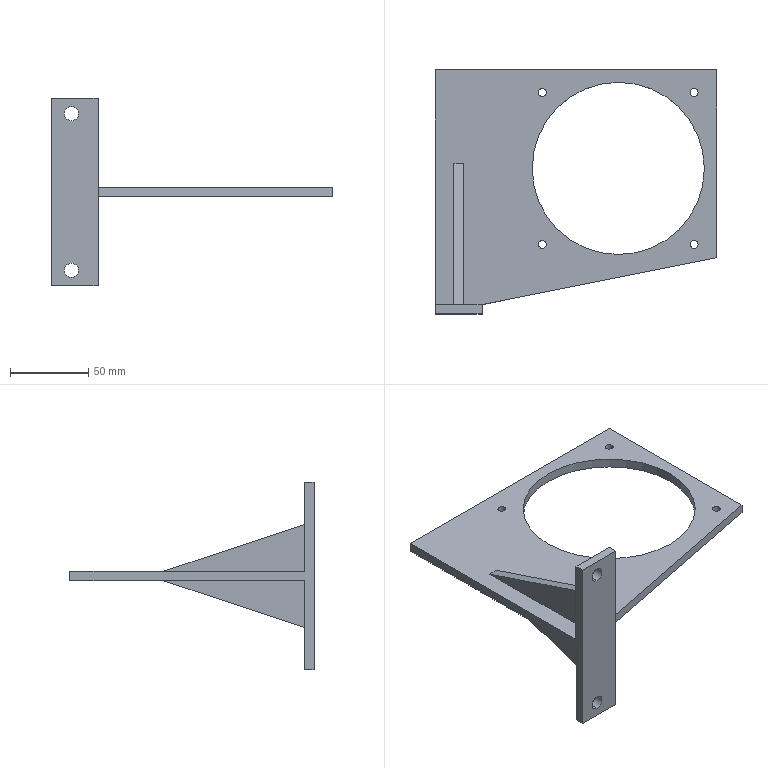Part | SolidWorks | features ICE 3, Extrusion 1 | 1 solid | 32 faces | box 180 x 156 x 120 mm | volume 128045 mm3 | plane 18 | cylinder 14 | commonest cylinder face diameters 5 x8 9 x4 110 x2
STEP:
#1=CARTESIAN_POINT('',(13.,-6.,48.5));
#2=VERTEX_POINT('',#1);
#3=CARTESIAN_POINT('',(13.,-6.,57.5));
#4=VERTEX_POINT('',#3);
#5=CARTESIAN_POINT('',(13.,-6.,53.));
#6=DIRECTION('',(0.,1.,0.));
#7=DIRECTION('',(0.,0.,1.));
#8=AXIS2_PLACEMENT_3D('',#5,#6,#7);
#9=CIRCLE('',#8,4.5);
#10=EDGE_CURVE('',#2,#4,#9,.T.);
#11=ORIENTED_EDGE('',*,*,#10,.F.);
#12=CARTESIAN_POINT('',(13.,0.,48.5));
#13=VERTEX_POINT('',#12);
#14=CARTESIAN_POINT('',(13.,-6.,48.5));
#15=DIRECTION('',(0.,1.,0.));
#16=VECTOR('',#15,1000.);
#17=LINE('',#14,#16);
#18=EDGE_CURVE('',#2,#13,#17,.T.);
#19=ORIENTED_EDGE('',*,*,#18,.T.);
#20=CARTESIAN_POINT('',(13.,0.,57.5));
#21=VERTEX_POINT('',#20);
#22=CARTESIAN_POINT('',(13.,0.,53.));
#23=DIRECTION('',(0.,1.,0.));
#24=DIRECTION('',(0.,0.,1.));
#25=AXIS2_PLACEMENT_3D('',#22,#23,#24);
#26=CIRCLE('',#25,4.5);
#27=EDGE_CURVE('',#13,#21,#26,.T.);
#28=ORIENTED_EDGE('',*,*,#27,.T.);
#29=CARTESIAN_POINT('',(13.,-6.,57.5));
#30=DIRECTION('',(0.,1.,0.));
#31=VECTOR('',#30,1000.);
#32=LINE('',#29,#31);
#33=EDGE_CURVE('',#4,#21,#32,.T.);
#34=ORIENTED_EDGE('',*,*,#33,.F.);
#35=EDGE_LOOP('',(#11,#19,#28,#34));
#36=FACE_OUTER_BOUND('',#35,.T.);
#37=CARTESIAN_POINT('',(13.,-6.,53.));
#38=DIRECTION('',(0.,1.,0.));
#39=DIRECTION('',(0.,0.,1.));
#40=AXIS2_PLACEMENT_3D('',#37,#38,#39);
#41=CYLINDRICAL_SURFACE('',#40,4.5);
#42=ADVANCED_FACE('',(#36),#41,.F.);
#43=CARTESIAN_POINT('',(13.,-6.,-51.5));
#44=VERTEX_POINT('',#43);
#45=CARTESIAN_POINT('',(13.,-6.,-42.5));
#46=VERTEX_POINT('',#45);
#47=CARTESIAN_POINT('',(13.,-6.,-47.));
#48=DIRECTION('',(0.,1.,0.));
#49=DIRECTION('',(0.,0.,1.));
#50=AXIS2_PLACEMENT_3D('',#47,#48,#49);
#51=CIRCLE('',#50,4.5);
#52=EDGE_CURVE('',#44,#46,#51,.T.);
#53=ORIENTED_EDGE('',*,*,#52,.F.);
#54=CARTESIAN_POINT('',(13.,0.,-51.5));
#55=VERTEX_POINT('',#54);
#56=CARTESIAN_POINT('',(13.,-6.,-51.5));
#57=DIRECTION('',(0.,1.,0.));
#58=VECTOR('',#57,1000.);
#59=LINE('',#56,#58);
#60=EDGE_CURVE('',#44,#55,#59,.T.);
#61=ORIENTED_EDGE('',*,*,#60,.T.);
#62=CARTESIAN_POINT('',(13.,0.,-42.5));
#63=VERTEX_POINT('',#62);
#64=CARTESIAN_POINT('',(13.,0.,-47.));
#65=DIRECTION('',(0.,1.,0.));
#66=DIRECTION('',(0.,0.,1.));
#67=AXIS2_PLACEMENT_3D('',#64,#65,#66);
#68=CIRCLE('',#67,4.5);
#69=EDGE_CURVE('',#55,#63,#68,.T.);
#70=ORIENTED_EDGE('',*,*,#69,.T.);
#71=CARTESIAN_POINT('',(13.,-6.,-42.5));
#72=DIRECTION('',(0.,1.,0.));
#73=VECTOR('',#72,1000.);
#74=LINE('',#71,#73);
#75=EDGE_CURVE('',#46,#63,#74,.T.);
#76=ORIENTED_EDGE('',*,*,#75,.F.);
#77=EDGE_LOOP('',(#53,#61,#70,#76));
#78=FACE_OUTER_BOUND('',#77,.T.);
#79=CARTESIAN_POINT('',(13.,-6.,-47.));
#80=DIRECTION('',(0.,1.,0.));
#81=DIRECTION('',(0.,0.,1.));
#82=AXIS2_PLACEMENT_3D('',#79,#80,#81);
#83=CYLINDRICAL_SURFACE('',#82,4.5);
#84=ADVANCED_FACE('',(#78),#83,.F.);
#85=CARTESIAN_POINT('',(62.,87.,6.));
#86=VERTEX_POINT('',#85);
#87=CARTESIAN_POINT('',(172.,87.,6.));
#88=VERTEX_POINT('',#87);
#89=CARTESIAN_POINT('',(117.,87.,6.));
#90=DIRECTION('',(0.,0.,1.));
#91=DIRECTION('',(1.,0.,0.));
#92=AXIS2_PLACEMENT_3D('',#89,#90,#91);
#93=CIRCLE('',#92,55.);
#94=EDGE_CURVE('',#86,#88,#93,.T.);
#95=ORIENTED_EDGE('',*,*,#94,.T.);
#96=CARTESIAN_POINT('',(172.,87.,0.));
#97=VERTEX_POINT('',#96);
#98=CARTESIAN_POINT('',(172.,87.,6.));
#99=DIRECTION('',(0.,0.,-1.));
#100=VECTOR('',#99,1000.);
#101=LINE('',#98,#100);
#102=EDGE_CURVE('',#88,#97,#101,.T.);
#103=ORIENTED_EDGE('',*,*,#102,.T.);
#104=CARTESIAN_POINT('',(62.,87.,0.));
#105=VERTEX_POINT('',#104);
#106=CARTESIAN_POINT('',(117.,87.,0.));
#107=DIRECTION('',(0.,0.,1.));
#108=DIRECTION('',(1.,0.,0.));
#109=AXIS2_PLACEMENT_3D('',#106,#107,#108);
#110=CIRCLE('',#109,55.);
#111=EDGE_CURVE('',#105,#97,#110,.T.);
#112=ORIENTED_EDGE('',*,*,#111,.F.);
#113=CARTESIAN_POINT('',(62.,87.,6.));
#114=DIRECTION('',(0.,0.,-1.));
#115=VECTOR('',#114,1000.);
#116=LINE('',#113,#115);
#117=EDGE_CURVE('',#86,#105,#116,.T.);
#118=ORIENTED_EDGE('',*,*,#117,.F.);
#119=EDGE_LOOP('',(#95,#103,#112,#118));
#120=FACE_OUTER_BOUND('',#119,.T.);
#121=CARTESIAN_POINT('',(117.,87.,6.));
#122=DIRECTION('',(0.,0.,-1.));
#123=DIRECTION('',(-1.,0.,0.));
#124=AXIS2_PLACEMENT_3D('',#121,#122,#123);
#125=CYLINDRICAL_SURFACE('',#124,55.);
#126=ADVANCED_FACE('',(#120),#125,.F.);
#127=CARTESIAN_POINT('',(66.,38.5,6.));
#128=VERTEX_POINT('',#127);
#129=CARTESIAN_POINT('',(71.,38.5,6.));
#130=VERTEX_POINT('',#129);
#131=CARTESIAN_POINT('',(68.5,38.5,6.));
#132=DIRECTION('',(0.,0.,1.));
#133=DIRECTION('',(1.,0.,0.));
#134=AXIS2_PLACEMENT_3D('',#131,#132,#133);
#135=CIRCLE('',#134,2.5);
#136=EDGE_CURVE('',#128,#130,#135,.T.);
#137=ORIENTED_EDGE('',*,*,#136,.T.);
#138=CARTESIAN_POINT('',(71.,38.5,0.));
#139=VERTEX_POINT('',#138);
#140=CARTESIAN_POINT('',(71.,38.5,6.));
#141=DIRECTION('',(0.,0.,-1.));
#142=VECTOR('',#141,1000.);
#143=LINE('',#140,#142);
#144=EDGE_CURVE('',#130,#139,#143,.T.);
#145=ORIENTED_EDGE('',*,*,#144,.T.);
#146=CARTESIAN_POINT('',(66.,38.5,0.));
#147=VERTEX_POINT('',#146);
#148=CARTESIAN_POINT('',(68.5,38.5,0.));
#149=DIRECTION('',(0.,0.,1.));
#150=DIRECTION('',(1.,0.,0.));
#151=AXIS2_PLACEMENT_3D('',#148,#149,#150);
#152=CIRCLE('',#151,2.5);
#153=EDGE_CURVE('',#147,#139,#152,.T.);
#154=ORIENTED_EDGE('',*,*,#153,.F.);
#155=CARTESIAN_POINT('',(66.,38.5,6.));
#156=DIRECTION('',(0.,0.,-1.));
#157=VECTOR('',#156,1000.);
#158=LINE('',#155,#157);
#159=EDGE_CURVE('',#128,#147,#158,.T.);
#160=ORIENTED_EDGE('',*,*,#159,.F.);
#161=EDGE_LOOP('',(#137,#145,#154,#160));
#162=FACE_OUTER_BOUND('',#161,.T.);
#163=CARTESIAN_POINT('',(68.5,38.5,6.));
#164=DIRECTION('',(0.,0.,-1.));
#165=DIRECTION('',(-1.,0.,0.));
#166=AXIS2_PLACEMENT_3D('',#163,#164,#165);
#167=CYLINDRICAL_SURFACE('',#166,2.5);
#168=ADVANCED_FACE('',(#162),#167,.F.);
#169=CARTESIAN_POINT('',(163.,38.5,6.));
#170=VERTEX_POINT('',#169);
#171=CARTESIAN_POINT('',(168.,38.5,6.));
#172=VERTEX_POINT('',#171);
#173=CARTESIAN_POINT('',(165.5,38.5,6.));
#174=DIRECTION('',(0.,0.,1.));
#175=DIRECTION('',(1.,0.,0.));
#176=AXIS2_PLACEMENT_3D('',#173,#174,#175);
#177=CIRCLE('',#176,2.5);
#178=EDGE_CURVE('',#170,#172,#177,.T.);
#179=ORIENTED_EDGE('',*,*,#178,.T.);
#180=CARTESIAN_POINT('',(168.,38.5,0.));
#181=VERTEX_POINT('',#180);
#182=CARTESIAN_POINT('',(168.,38.5,6.));
#183=DIRECTION('',(0.,0.,-1.));
#184=VECTOR('',#183,1000.);
#185=LINE('',#182,#184);
#186=EDGE_CURVE('',#172,#181,#185,.T.);
#187=ORIENTED_EDGE('',*,*,#186,.T.);
#188=CARTESIAN_POINT('',(163.,38.5,0.));
#189=VERTEX_POINT('',#188);
#190=CARTESIAN_POINT('',(165.5,38.5,0.));
#191=DIRECTION('',(0.,0.,1.));
#192=DIRECTION('',(1.,0.,0.));
#193=AXIS2_PLACEMENT_3D('',#190,#191,#192);
#194=CIRCLE('',#193,2.5);
#195=EDGE_CURVE('',#189,#181,#194,.T.);
#196=ORIENTED_EDGE('',*,*,#195,.F.);
#197=CARTESIAN_POINT('',(163.,38.5,6.));
#198=DIRECTION('',(0.,0.,-1.));
#199=VECTOR('',#198,1000.);
#200=LINE('',#197,#199);
#201=EDGE_CURVE('',#170,#189,#200,.T.);
#202=ORIENTED_EDGE('',*,*,#201,.F.);
#203=EDGE_LOOP('',(#179,#187,#196,#202));
#204=FACE_OUTER_BOUND('',#203,.T.);
#205=CARTESIAN_POINT('',(165.5,38.5,6.));
#206=DIRECTION('',(0.,0.,-1.));
#207=DIRECTION('',(-1.,0.,0.));
#208=AXIS2_PLACEMENT_3D('',#205,#206,#207);
#209=CYLINDRICAL_SURFACE('',#208,2.5);
#210=ADVANCED_FACE('',(#204),#209,.F.);
#211=CARTESIAN_POINT('',(66.,135.5,6.));
#212=VERTEX_POINT('',#211);
#213=CARTESIAN_POINT('',(71.,135.5,6.));
#214=VERTEX_POINT('',#213);
#215=CARTESIAN_POINT('',(68.5,135.5,6.));
#216=DIRECTION('',(0.,0.,1.));
#217=DIRECTION('',(1.,0.,0.));
#218=AXIS2_PLACEMENT_3D('',#215,#216,#217);
#219=CIRCLE('',#218,2.5);
#220=EDGE_CURVE('',#212,#214,#219,.T.);
#221=ORIENTED_EDGE('',*,*,#220,.T.);
#222=CARTESIAN_POINT('',(71.,135.5,0.));
#223=VERTEX_POINT('',#222);
#224=CARTESIAN_POINT('',(71.,135.5,6.));
#225=DIRECTION('',(0.,0.,-1.));
#226=VECTOR('',#225,1000.);
#227=LINE('',#224,#226);
#228=EDGE_CURVE('',#214,#223,#227,.T.);
#229=ORIENTED_EDGE('',*,*,#228,.T.);
#230=CARTESIAN_POINT('',(66.,135.5,0.));
#231=VERTEX_POINT('',#230);
#232=CARTESIAN_POINT('',(68.5,135.5,0.));
#233=DIRECTION('',(0.,0.,1.));
#234=DIRECTION('',(1.,0.,0.));
#235=AXIS2_PLACEMENT_3D('',#232,#233,#234);
#236=CIRCLE('',#235,2.5);
#237=EDGE_CURVE('',#231,#223,#236,.T.);
#238=ORIENTED_EDGE('',*,*,#237,.F.);
#239=CARTESIAN_POINT('',(66.,135.5,6.));
#240=DIRECTION('',(0.,0.,-1.));
#241=VECTOR('',#240,1000.);
#242=LINE('',#239,#241);
#243=EDGE_CURVE('',#212,#231,#242,.T.);
#244=ORIENTED_EDGE('',*,*,#243,.F.);
#245=EDGE_LOOP('',(#221,#229,#238,#244));
#246=FACE_OUTER_BOUND('',#245,.T.);
#247=CARTESIAN_POINT('',(68.5,135.5,6.));
#248=DIRECTION('',(0.,0.,-1.));
#249=DIRECTION('',(-1.,0.,0.));
#250=AXIS2_PLACEMENT_3D('',#247,#248,#249);
#251=CYLINDRICAL_SURFACE('',#250,2.5);
#252=ADVANCED_FACE('',(#246),#251,.F.);
#253=CARTESIAN_POINT('',(163.,135.5,6.));
#254=VERTEX_POINT('',#253);
#255=CARTESIAN_POINT('',(168.,135.5,6.));
#256=VERTEX_POINT('',#255);
#257=CARTESIAN_POINT('',(165.5,135.5,6.));
#258=DIRECTION('',(0.,0.,1.));
#259=DIRECTION('',(1.,0.,0.));
#260=AXIS2_PLACEMENT_3D('',#257,#258,#259);
#261=CIRCLE('',#260,2.5);
#262=EDGE_CURVE('',#254,#256,#261,.T.);
#263=ORIENTED_EDGE('',*,*,#262,.T.);
#264=CARTESIAN_POINT('',(168.,135.5,0.));
#265=VERTEX_POINT('',#264);
#266=CARTESIAN_POINT('',(168.,135.5,6.));
#267=DIRECTION('',(0.,0.,-1.));
#268=VECTOR('',#267,1000.);
#269=LINE('',#266,#268);
#270=EDGE_CURVE('',#256,#265,#269,.T.);
#271=ORIENTED_EDGE('',*,*,#270,.T.);
#272=CARTESIAN_POINT('',(163.,135.5,0.));
#273=VERTEX_POINT('',#272);
#274=CARTESIAN_POINT('',(165.5,135.5,0.));
#275=DIRECTION('',(0.,0.,1.));
#276=DIRECTION('',(1.,0.,0.));
#277=AXIS2_PLACEMENT_3D('',#274,#275,#276);
#278=CIRCLE('',#277,2.5);
#279=EDGE_CURVE('',#273,#265,#278,.T.);
#280=ORIENTED_EDGE('',*,*,#279,.F.);
#281=CARTESIAN_POINT('',(163.,135.5,6.));
#282=DIRECTION('',(0.,0.,-1.));
#283=VECTOR('',#282,1000.);
#284=LINE('',#281,#283);
#285=EDGE_CURVE('',#254,#273,#284,.T.);
#286=ORIENTED_EDGE('',*,*,#285,.F.);
#287=EDGE_LOOP('',(#263,#271,#280,#286));
#288=FACE_OUTER_BOUND('',#287,.T.);
#289=CARTESIAN_POINT('',(165.5,135.5,6.));
#290=DIRECTION('',(0.,0.,-1.));
#291=DIRECTION('',(-1.,0.,0.));
#292=AXIS2_PLACEMENT_3D('',#289,#290,#291);
#293=CYLINDRICAL_SURFACE('',#292,2.5);
#294=ADVANCED_FACE('',(#288),#293,.F.);
#295=ORIENTED_EDGE('',*,*,#136,.F.);
#296=CARTESIAN_POINT('',(68.5,38.5,6.));
#297=DIRECTION('',(0.,0.,1.));
#298=DIRECTION('',(1.,0.,0.));
#299=AXIS2_PLACEMENT_3D('',#296,#297,#298);
#300=CIRCLE('',#299,2.5);
#301=EDGE_CURVE('',#130,#128,#300,.T.);
#302=ORIENTED_EDGE('',*,*,#301,.F.);
#303=EDGE_LOOP('',(#295,#302));
#304=FACE_BOUND('',#303,.T.);
#305=ORIENTED_EDGE('',*,*,#220,.F.);
#306=CARTESIAN_POINT('',(68.5,135.5,6.));
#307=DIRECTION('',(0.,0.,1.));
#308=DIRECTION('',(1.,0.,0.));
#309=AXIS2_PLACEMENT_3D('',#306,#307,#308);
#310=CIRCLE('',#309,2.5);
#311=EDGE_CURVE('',#214,#212,#310,.T.);
#312=ORIENTED_EDGE('',*,*,#311,.F.);
#313=EDGE_LOOP('',(#305,#312));
#314=FACE_BOUND('',#313,.T.);
#315=CARTESIAN_POINT('',(18.,90.,6.));
#316=VERTEX_POINT('',#315);
#317=CARTESIAN_POINT('',(12.,90.,6.));
#318=VERTEX_POINT('',#317);
#319=CARTESIAN_POINT('',(18.,90.,6.));
#320=DIRECTION('',(-1.,0.,0.));
#321=VECTOR('',#320,1000.);
#322=LINE('',#319,#321);
#323=EDGE_CURVE('',#316,#318,#322,.T.);
#324=ORIENTED_EDGE('',*,*,#323,.F.);
#325=CARTESIAN_POINT('',(18.,0.,6.));
#326=VERTEX_POINT('',#325);
#327=CARTESIAN_POINT('',(18.,0.,6.));
#328=DIRECTION('',(0.,-1.,0.));
#329=VECTOR('',#328,1000.);
#330=LINE('',#327,#329);
#331=EDGE_CURVE('',#316,#326,#330,.T.);
#332=ORIENTED_EDGE('',*,*,#331,.T.);
#333=CARTESIAN_POINT('',(30.,0.,6.));
#334=VERTEX_POINT('',#333);
#335=CARTESIAN_POINT('',(0.,0.,6.));
#336=DIRECTION('',(1.,0.,0.));
#337=VECTOR('',#336,1000.);
#338=LINE('',#335,#337);
#339=EDGE_CURVE('',#326,#334,#338,.T.);
#340=ORIENTED_EDGE('',*,*,#339,.T.);
#341=CARTESIAN_POINT('',(180.,30.,6.));
#342=VERTEX_POINT('',#341);
#343=CARTESIAN_POINT('',(180.,30.,6.));
#344=DIRECTION('',(0.9806,0.1961,0.));
#345=VECTOR('',#344,1000.);
#346=LINE('',#343,#345);
#347=EDGE_CURVE('',#334,#342,#346,.T.);
#348=ORIENTED_EDGE('',*,*,#347,.T.);
#349=CARTESIAN_POINT('',(180.,150.,6.));
#350=VERTEX_POINT('',#349);
#351=CARTESIAN_POINT('',(180.,30.,6.));
#352=DIRECTION('',(0.,1.,0.));
#353=VECTOR('',#352,1000.);
#354=LINE('',#351,#353);
#355=EDGE_CURVE('',#342,#350,#354,.T.);
#356=ORIENTED_EDGE('',*,*,#355,.T.);
#357=CARTESIAN_POINT('',(0.,150.,6.));
#358=VERTEX_POINT('',#357);
#359=CARTESIAN_POINT('',(0.,150.,6.));
#360=DIRECTION('',(-1.,0.,0.));
#361=VECTOR('',#360,1000.);
#362=LINE('',#359,#361);
#363=EDGE_CURVE('',#350,#358,#362,.T.);
#364=ORIENTED_EDGE('',*,*,#363,.T.);
#365=CARTESIAN_POINT('',(0.,0.,6.));
#366=VERTEX_POINT('',#365);
#367=CARTESIAN_POINT('',(0.,0.,6.));
#368=DIRECTION('',(0.,-1.,0.));
#369=VECTOR('',#368,1000.);
#370=LINE('',#367,#369);
#371=EDGE_CURVE('',#358,#366,#370,.T.);
#372=ORIENTED_EDGE('',*,*,#371,.T.);
#373=CARTESIAN_POINT('',(12.,0.,6.));
#374=VERTEX_POINT('',#373);
#375=CARTESIAN_POINT('',(0.,0.,6.));
#376=DIRECTION('',(1.,0.,0.));
#377=VECTOR('',#376,1000.);
#378=LINE('',#375,#377);
#379=EDGE_CURVE('',#366,#374,#378,.T.);
#380=ORIENTED_EDGE('',*,*,#379,.T.);
#381=CARTESIAN_POINT('',(12.,0.,6.));
#382=DIRECTION('',(0.,-1.,0.));
#383=VECTOR('',#382,1000.);
#384=LINE('',#381,#383);
#385=EDGE_CURVE('',#318,#374,#384,.T.);
#386=ORIENTED_EDGE('',*,*,#385,.F.);
#387=EDGE_LOOP('',(#324,#332,#340,#348,#356,#364,#372,#380,#386));
#388=FACE_OUTER_BOUND('',#387,.T.);
#389=ORIENTED_EDGE('',*,*,#262,.F.);
#390=CARTESIAN_POINT('',(165.5,135.5,6.));
#391=DIRECTION('',(0.,0.,1.));
#392=DIRECTION('',(1.,0.,0.));
#393=AXIS2_PLACEMENT_3D('',#390,#391,#392);
#394=CIRCLE('',#393,2.5);
#395=EDGE_CURVE('',#256,#254,#394,.T.);
#396=ORIENTED_EDGE('',*,*,#395,.F.);
#397=EDGE_LOOP('',(#389,#396));
#398=FACE_BOUND('',#397,.T.);
#399=ORIENTED_EDGE('',*,*,#178,.F.);
#400=CARTESIAN_POINT('',(165.5,38.5,6.));
#401=DIRECTION('',(0.,0.,1.));
#402=DIRECTION('',(1.,0.,0.));
#403=AXIS2_PLACEMENT_3D('',#400,#401,#402);
#404=CIRCLE('',#403,2.5);
#405=EDGE_CURVE('',#172,#170,#404,.T.);
#406=ORIENTED_EDGE('',*,*,#405,.F.);
#407=EDGE_LOOP('',(#399,#406));
#408=FACE_BOUND('',#407,.T.);
#409=ORIENTED_EDGE('',*,*,#94,.F.);
#410=CARTESIAN_POINT('',(117.,87.,6.));
#411=DIRECTION('',(0.,0.,1.));
#412=DIRECTION('',(1.,0.,0.));
#413=AXIS2_PLACEMENT_3D('',#410,#411,#412);
#414=CIRCLE('',#413,55.);
#415=EDGE_CURVE('',#88,#86,#414,.T.);
#416=ORIENTED_EDGE('',*,*,#415,.F.);
#417=EDGE_LOOP('',(#409,#416));
#418=FACE_BOUND('',#417,.T.);
#419=CARTESIAN_POINT('',(0.,150.,6.));
#420=DIRECTION('',(0.,0.,-1.));
#421=DIRECTION('',(-1.,0.,0.));
#422=AXIS2_PLACEMENT_3D('',#419,#420,#421);
#423=PLANE('',#422);
#424=ADVANCED_FACE('',(#304,#314,#388,#398,#408,#418),#423,.F.);
#425=CARTESIAN_POINT('',(18.,0.,0.));
#426=VERTEX_POINT('',#425);
#427=CARTESIAN_POINT('',(18.,90.,0.));
#428=VERTEX_POINT('',#427);
#429=CARTESIAN_POINT('',(18.,0.,0.));
#430=DIRECTION('',(0.,1.,0.));
#431=VECTOR('',#430,1000.);
#432=LINE('',#429,#431);
#433=EDGE_CURVE('',#426,#428,#432,.T.);
#434=ORIENTED_EDGE('',*,*,#433,.T.);
#435=CARTESIAN_POINT('',(12.,90.,0.));
#436=VERTEX_POINT('',#435);
#437=CARTESIAN_POINT('',(18.,90.,0.));
#438=DIRECTION('',(-1.,0.,0.));
#439=VECTOR('',#438,1000.);
#440=LINE('',#437,#439);
#441=EDGE_CURVE('',#428,#436,#440,.T.);
#442=ORIENTED_EDGE('',*,*,#441,.T.);
#443=CARTESIAN_POINT('',(12.,0.,0.));
#444=VERTEX_POINT('',#443);
#445=CARTESIAN_POINT('',(12.,0.,0.));
#446=DIRECTION('',(0.,1.,0.));
#447=VECTOR('',#446,1000.);
#448=LINE('',#445,#447);
#449=EDGE_CURVE('',#444,#436,#448,.T.);
#450=ORIENTED_EDGE('',*,*,#449,.F.);
#451=CARTESIAN_POINT('',(0.,0.,0.));
#452=VERTEX_POINT('',#451);
#453=CARTESIAN_POINT('',(0.,0.,0.));
#454=DIRECTION('',(1.,0.,0.));
#455=VECTOR('',#454,1000.);
#456=LINE('',#453,#455);
#457=EDGE_CURVE('',#452,#444,#456,.T.);
#458=ORIENTED_EDGE('',*,*,#457,.F.);
#459=CARTESIAN_POINT('',(0.,150.,0.));
#460=VERTEX_POINT('',#459);
#461=CARTESIAN_POINT('',(0.,0.,0.));
#462=DIRECTION('',(0.,-1.,0.));
#463=VECTOR('',#462,1000.);
#464=LINE('',#461,#463);
#465=EDGE_CURVE('',#460,#452,#464,.T.);
#466=ORIENTED_EDGE('',*,*,#465,.F.);
#467=CARTESIAN_POINT('',(180.,150.,0.));
#468=VERTEX_POINT('',#467);
#469=CARTESIAN_POINT('',(0.,150.,0.));
#470=DIRECTION('',(-1.,0.,0.));
#471=VECTOR('',#470,1000.);
#472=LINE('',#469,#471);
#473=EDGE_CURVE('',#468,#460,#472,.T.);
#474=ORIENTED_EDGE('',*,*,#473,.F.);
#475=CARTESIAN_POINT('',(180.,30.,0.));
#476=VERTEX_POINT('',#475);
#477=CARTESIAN_POINT('',(180.,30.,0.));
#478=DIRECTION('',(0.,1.,0.));
#479=VECTOR('',#478,1000.);
#480=LINE('',#477,#479);
#481=EDGE_CURVE('',#476,#468,#480,.T.);
#482=ORIENTED_EDGE('',*,*,#481,.F.);
#483=CARTESIAN_POINT('',(30.,0.,0.));
#484=VERTEX_POINT('',#483);
#485=CARTESIAN_POINT('',(180.,30.,0.));
#486=DIRECTION('',(0.9806,0.1961,0.));
#487=VECTOR('',#486,1000.);
#488=LINE('',#485,#487);
#489=EDGE_CURVE('',#484,#476,#488,.T.);
#490=ORIENTED_EDGE('',*,*,#489,.F.);
#491=CARTESIAN_POINT('',(0.,0.,0.));
#492=DIRECTION('',(1.,0.,0.));
#493=VECTOR('',#492,1000.);
#494=LINE('',#491,#493);
#495=EDGE_CURVE('',#426,#484,#494,.T.);
#496=ORIENTED_EDGE('',*,*,#495,.F.);
#497=EDGE_LOOP('',(#434,#442,#450,#458,#466,#474,#482,#490,#496));
#498=FACE_OUTER_BOUND('',#497,.T.);
#499=ORIENTED_EDGE('',*,*,#153,.T.);
#500=CARTESIAN_POINT('',(68.5,38.5,0.));
#501=DIRECTION('',(0.,0.,1.));
#502=DIRECTION('',(1.,0.,0.));
#503=AXIS2_PLACEMENT_3D('',#500,#501,#502);
#504=CIRCLE('',#503,2.5);
#505=EDGE_CURVE('',#139,#147,#504,.T.);
#506=ORIENTED_EDGE('',*,*,#505,.T.);
#507=EDGE_LOOP('',(#499,#506));
#508=FACE_BOUND('',#507,.T.);
#509=ORIENTED_EDGE('',*,*,#237,.T.);
#510=CARTESIAN_POINT('',(68.5,135.5,0.));
#511=DIRECTION('',(0.,0.,1.));
#512=DIRECTION('',(1.,0.,0.));
#513=AXIS2_PLACEMENT_3D('',#510,#511,#512);
#514=CIRCLE('',#513,2.5);
#515=EDGE_CURVE('',#223,#231,#514,.T.);
#516=ORIENTED_EDGE('',*,*,#515,.T.);
#517=EDGE_LOOP('',(#509,#516));
#518=FACE_BOUND('',#517,.T.);
#519=ORIENTED_EDGE('',*,*,#279,.T.);
#520=CARTESIAN_POINT('',(165.5,135.5,0.));
#521=DIRECTION('',(0.,0.,1.));
#522=DIRECTION('',(1.,0.,0.));
#523=AXIS2_PLACEMENT_3D('',#520,#521,#522);
#524=CIRCLE('',#523,2.5);
#525=EDGE_CURVE('',#265,#273,#524,.T.);
#526=ORIENTED_EDGE('',*,*,#525,.T.);
#527=EDGE_LOOP('',(#519,#526));
#528=FACE_BOUND('',#527,.T.);
#529=ORIENTED_EDGE('',*,*,#195,.T.);
#530=CARTESIAN_POINT('',(165.5,38.5,0.));
#531=DIRECTION('',(0.,0.,1.));
#532=DIRECTION('',(1.,0.,0.));
#533=AXIS2_PLACEMENT_3D('',#530,#531,#532);
#534=CIRCLE('',#533,2.5);
#535=EDGE_CURVE('',#181,#189,#534,.T.);
#536=ORIENTED_EDGE('',*,*,#535,.T.);
#537=EDGE_LOOP('',(#529,#536));
#538=FACE_BOUND('',#537,.T.);
#539=ORIENTED_EDGE('',*,*,#111,.T.);
#540=CARTESIAN_POINT('',(117.,87.,0.));
#541=DIRECTION('',(0.,0.,1.));
#542=DIRECTION('',(1.,0.,0.));
#543=AXIS2_PLACEMENT_3D('',#540,#541,#542);
#544=CIRCLE('',#543,55.);
#545=EDGE_CURVE('',#97,#105,#544,.T.);
#546=ORIENTED_EDGE('',*,*,#545,.T.);
#547=EDGE_LOOP('',(#539,#546));
#548=FACE_BOUND('',#547,.T.);
#549=CARTESIAN_POINT('',(0.,150.,0.));
#550=DIRECTION('',(0.,0.,-1.));
#551=DIRECTION('',(-1.,0.,0.));
#552=AXIS2_PLACEMENT_3D('',#549,#550,#551);
#553=PLANE('',#552);
#554=ADVANCED_FACE('',(#498,#508,#518,#528,#538,#548),#553,.T.);
#555=ORIENTED_EDGE('',*,*,#465,.T.);
#556=CARTESIAN_POINT('',(0.,0.,-57.));
#557=VERTEX_POINT('',#556);
#558=CARTESIAN_POINT('',(0.,0.,63.));
#559=DIRECTION('',(0.,0.,-1.));
#560=VECTOR('',#559,1000.);
#561=LINE('',#558,#560);
#562=EDGE_CURVE('',#452,#557,#561,.T.);
#563=ORIENTED_EDGE('',*,*,#562,.T.);
#564=CARTESIAN_POINT('',(0.,-6.,-57.));
#565=VERTEX_POINT('',#564);
#566=CARTESIAN_POINT('',(0.,-6.,-57.));
#567=DIRECTION('',(0.,1.,0.));
#568=VECTOR('',#567,1000.);
#569=LINE('',#566,#568);
#570=EDGE_CURVE('',#565,#557,#569,.T.);
#571=ORIENTED_EDGE('',*,*,#570,.F.);
#572=CARTESIAN_POINT('',(0.,-6.,63.));
#573=VERTEX_POINT('',#572);
#574=CARTESIAN_POINT('',(0.,-6.,63.));
#575=DIRECTION('',(0.,0.,-1.));
#576=VECTOR('',#575,1000.);
#577=LINE('',#574,#576);
#578=EDGE_CURVE('',#573,#565,#577,.T.);
#579=ORIENTED_EDGE('',*,*,#578,.F.);
#580=CARTESIAN_POINT('',(0.,0.,63.));
#581=VERTEX_POINT('',#580);
#582=CARTESIAN_POINT('',(0.,-6.,63.));
#583=DIRECTION('',(0.,1.,0.));
#584=VECTOR('',#583,1000.);
#585=LINE('',#582,#584);
#586=EDGE_CURVE('',#573,#581,#585,.T.);
#587=ORIENTED_EDGE('',*,*,#586,.T.);
#588=CARTESIAN_POINT('',(0.,0.,63.));
#589=DIRECTION('',(0.,0.,-1.));
#590=VECTOR('',#589,1000.);
#591=LINE('',#588,#590);
#592=EDGE_CURVE('',#581,#366,#591,.T.);
#593=ORIENTED_EDGE('',*,*,#592,.T.);
#594=ORIENTED_EDGE('',*,*,#371,.F.);
#595=CARTESIAN_POINT('',(0.,150.,6.));
#596=DIRECTION('',(0.,0.,-1.));
#597=VECTOR('',#596,1000.);
#598=LINE('',#595,#597);
#599=EDGE_CURVE('',#358,#460,#598,.T.);
#600=ORIENTED_EDGE('',*,*,#599,.T.);
#601=EDGE_LOOP('',(#555,#563,#571,#579,#587,#593,#594,#600));
#602=FACE_OUTER_BOUND('',#601,.T.);
#603=CARTESIAN_POINT('',(0.,0.,6.));
#604=DIRECTION('',(1.,0.,0.));
#605=DIRECTION('',(0.,1.,0.));
#606=AXIS2_PLACEMENT_3D('',#603,#604,#605);
#607=PLANE('',#606);
#608=ADVANCED_FACE('',(#602),#607,.F.);
#609=ORIENTED_EDGE('',*,*,#489,.T.);
#610=CARTESIAN_POINT('',(180.,30.,6.));
#611=DIRECTION('',(0.,0.,-1.));
#612=VECTOR('',#611,1000.);
#613=LINE('',#610,#612);
#614=EDGE_CURVE('',#342,#476,#613,.T.);
#615=ORIENTED_EDGE('',*,*,#614,.F.);
#616=ORIENTED_EDGE('',*,*,#347,.F.);
#617=CARTESIAN_POINT('',(30.,0.,6.));
#618=DIRECTION('',(0.,0.,-1.));
#619=VECTOR('',#618,1000.);
#620=LINE('',#617,#619);
#621=EDGE_CURVE('',#334,#484,#620,.T.);
#622=ORIENTED_EDGE('',*,*,#621,.T.);
#623=EDGE_LOOP('',(#609,#615,#616,#622));
#624=FACE_OUTER_BOUND('',#623,.T.);
#625=CARTESIAN_POINT('',(180.,30.,6.));
#626=DIRECTION('',(-0.1961,0.9806,0.));
#627=DIRECTION('',(-0.9806,-0.1961,0.));
#628=AXIS2_PLACEMENT_3D('',#625,#626,#627);
#629=PLANE('',#628);
#630=ADVANCED_FACE('',(#624),#629,.F.);
#631=ORIENTED_EDGE('',*,*,#481,.T.);
#632=CARTESIAN_POINT('',(180.,150.,6.));
#633=DIRECTION('',(0.,0.,-1.));
#634=VECTOR('',#633,1000.);
#635=LINE('',#632,#634);
#636=EDGE_CURVE('',#350,#468,#635,.T.);
#637=ORIENTED_EDGE('',*,*,#636,.F.);
#638=ORIENTED_EDGE('',*,*,#355,.F.);
#639=ORIENTED_EDGE('',*,*,#614,.T.);
#640=EDGE_LOOP('',(#631,#637,#638,#639));
#641=FACE_OUTER_BOUND('',#640,.T.);
#642=CARTESIAN_POINT('',(180.,30.,6.));
#643=DIRECTION('',(-1.,0.,0.));
#644=DIRECTION('',(0.,0.,1.));
#645=AXIS2_PLACEMENT_3D('',#642,#643,#644);
#646=PLANE('',#645);
#647=ADVANCED_FACE('',(#641),#646,.F.);
#648=ORIENTED_EDGE('',*,*,#473,.T.);
#649=ORIENTED_EDGE('',*,*,#599,.F.);
#650=ORIENTED_EDGE('',*,*,#363,.F.);
#651=ORIENTED_EDGE('',*,*,#636,.T.);
#652=EDGE_LOOP('',(#648,#649,#650,#651));
#653=FACE_OUTER_BOUND('',#652,.T.);
#654=CARTESIAN_POINT('',(0.,150.,6.));
#655=DIRECTION('',(0.,-1.,0.));
#656=DIRECTION('',(0.,0.,-1.));
#657=AXIS2_PLACEMENT_3D('',#654,#655,#656);
#658=PLANE('',#657);
#659=ADVANCED_FACE('',(#653),#658,.F.);
#660=ORIENTED_EDGE('',*,*,#270,.F.);
#661=ORIENTED_EDGE('',*,*,#395,.T.);
#662=ORIENTED_EDGE('',*,*,#285,.T.);
#663=ORIENTED_EDGE('',*,*,#525,.F.);
#664=EDGE_LOOP('',(#660,#661,#662,#663));
#665=FACE_OUTER_BOUND('',#664,.T.);
#666=CARTESIAN_POINT('',(165.5,135.5,6.));
#667=DIRECTION('',(0.,0.,-1.));
#668=DIRECTION('',(-1.,0.,0.));
#669=AXIS2_PLACEMENT_3D('',#666,#667,#668);
#670=CYLINDRICAL_SURFACE('',#669,2.5);
#671=ADVANCED_FACE('',(#665),#670,.F.);
#672=ORIENTED_EDGE('',*,*,#228,.F.);
#673=ORIENTED_EDGE('',*,*,#311,.T.);
#674=ORIENTED_EDGE('',*,*,#243,.T.);
#675=ORIENTED_EDGE('',*,*,#515,.F.);
#676=EDGE_LOOP('',(#672,#673,#674,#675));
#677=FACE_OUTER_BOUND('',#676,.T.);
#678=CARTESIAN_POINT('',(68.5,135.5,6.));
#679=DIRECTION('',(0.,0.,-1.));
#680=DIRECTION('',(-1.,0.,0.));
#681=AXIS2_PLACEMENT_3D('',#678,#679,#680);
#682=CYLINDRICAL_SURFACE('',#681,2.5);
#683=ADVANCED_FACE('',(#677),#682,.F.);
#684=ORIENTED_EDGE('',*,*,#186,.F.);
#685=ORIENTED_EDGE('',*,*,#405,.T.);
#686=ORIENTED_EDGE('',*,*,#201,.T.);
#687=ORIENTED_EDGE('',*,*,#535,.F.);
#688=EDGE_LOOP('',(#684,#685,#686,#687));
#689=FACE_OUTER_BOUND('',#688,.T.);
#690=CARTESIAN_POINT('',(165.5,38.5,6.));
#691=DIRECTION('',(0.,0.,-1.));
#692=DIRECTION('',(-1.,0.,0.));
#693=AXIS2_PLACEMENT_3D('',#690,#691,#692);
#694=CYLINDRICAL_SURFACE('',#693,2.5);
#695=ADVANCED_FACE('',(#689),#694,.F.);
#696=ORIENTED_EDGE('',*,*,#144,.F.);
#697=ORIENTED_EDGE('',*,*,#301,.T.);
#698=ORIENTED_EDGE('',*,*,#159,.T.);
#699=ORIENTED_EDGE('',*,*,#505,.F.);
#700=EDGE_LOOP('',(#696,#697,#698,#699));
#701=FACE_OUTER_BOUND('',#700,.T.);
#702=CARTESIAN_POINT('',(68.5,38.5,6.));
#703=DIRECTION('',(0.,0.,-1.));
#704=DIRECTION('',(-1.,0.,0.));
#705=AXIS2_PLACEMENT_3D('',#702,#703,#704);
#706=CYLINDRICAL_SURFACE('',#705,2.5);
#707=ADVANCED_FACE('',(#701),#706,.F.);
#708=ORIENTED_EDGE('',*,*,#102,.F.);
#709=ORIENTED_EDGE('',*,*,#415,.T.);
#710=ORIENTED_EDGE('',*,*,#117,.T.);
#711=ORIENTED_EDGE('',*,*,#545,.F.);
#712=EDGE_LOOP('',(#708,#709,#710,#711));
#713=FACE_OUTER_BOUND('',#712,.T.);
#714=CARTESIAN_POINT('',(117.,87.,6.));
#715=DIRECTION('',(0.,0.,-1.));
#716=DIRECTION('',(-1.,0.,0.));
#717=AXIS2_PLACEMENT_3D('',#714,#715,#716);
#718=CYLINDRICAL_SURFACE('',#717,55.);
#719=ADVANCED_FACE('',(#713),#718,.F.);
#720=CARTESIAN_POINT('',(13.,0.,-47.));
#721=DIRECTION('',(0.,1.,0.));
#722=DIRECTION('',(0.,0.,1.));
#723=AXIS2_PLACEMENT_3D('',#720,#721,#722);
#724=CIRCLE('',#723,4.5);
#725=EDGE_CURVE('',#63,#55,#724,.T.);
#726=ORIENTED_EDGE('',*,*,#725,.F.);
#727=ORIENTED_EDGE('',*,*,#69,.F.);
#728=EDGE_LOOP('',(#726,#727));
#729=FACE_BOUND('',#728,.T.);
#730=CARTESIAN_POINT('',(18.,0.,-30.));
#731=VERTEX_POINT('',#730);
#732=CARTESIAN_POINT('',(12.,0.,-30.));
#733=VERTEX_POINT('',#732);
#734=CARTESIAN_POINT('',(18.,0.,-30.));
#735=DIRECTION('',(-1.,0.,0.));
#736=VECTOR('',#735,1000.);
#737=LINE('',#734,#736);
#738=EDGE_CURVE('',#731,#733,#737,.T.);
#739=ORIENTED_EDGE('',*,*,#738,.F.);
#740=CARTESIAN_POINT('',(18.,0.,-30.));
#741=DIRECTION('',(0.,0.,1.));
#742=VECTOR('',#741,1000.);
#743=LINE('',#740,#742);
#744=EDGE_CURVE('',#731,#426,#743,.T.);
#745=ORIENTED_EDGE('',*,*,#744,.T.);
#746=ORIENTED_EDGE('',*,*,#495,.T.);
#747=CARTESIAN_POINT('',(30.,0.,-57.));
#748=VERTEX_POINT('',#747);
#749=CARTESIAN_POINT('',(30.,0.,63.));
#750=DIRECTION('',(0.,0.,1.));
#751=VECTOR('',#750,1000.);
#752=LINE('',#749,#751);
#753=EDGE_CURVE('',#748,#484,#752,.T.);
#754=ORIENTED_EDGE('',*,*,#753,.F.);
#755=CARTESIAN_POINT('',(0.,0.,-57.));
#756=DIRECTION('',(1.,0.,0.));
#757=VECTOR('',#756,1000.);
#758=LINE('',#755,#757);
#759=EDGE_CURVE('',#557,#748,#758,.T.);
#760=ORIENTED_EDGE('',*,*,#759,.F.);
#761=ORIENTED_EDGE('',*,*,#562,.F.);
#762=ORIENTED_EDGE('',*,*,#457,.T.);
#763=CARTESIAN_POINT('',(12.,0.,-30.));
#764=DIRECTION('',(0.,0.,1.));
#765=VECTOR('',#764,1000.);
#766=LINE('',#763,#765);
#767=EDGE_CURVE('',#733,#444,#766,.T.);
#768=ORIENTED_EDGE('',*,*,#767,.F.);
#769=EDGE_LOOP('',(#739,#745,#746,#754,#760,#761,#762,#768));
#770=FACE_OUTER_BOUND('',#769,.T.);
#771=CARTESIAN_POINT('',(0.,0.,-57.));
#772=DIRECTION('',(0.,-1.,0.));
#773=DIRECTION('',(0.,0.,-1.));
#774=AXIS2_PLACEMENT_3D('',#771,#772,#773);
#775=PLANE('',#774);
#776=ADVANCED_FACE('',(#729,#770),#775,.F.);
#777=ORIENTED_EDGE('',*,*,#759,.T.);
#778=CARTESIAN_POINT('',(30.,-6.,-57.));
#779=VERTEX_POINT('',#778);
#780=CARTESIAN_POINT('',(30.,-6.,-57.));
#781=DIRECTION('',(0.,1.,0.));
#782=VECTOR('',#781,1000.);
#783=LINE('',#780,#782);
#784=EDGE_CURVE('',#779,#748,#783,.T.);
#785=ORIENTED_EDGE('',*,*,#784,.F.);
#786=CARTESIAN_POINT('',(0.,-6.,-57.));
#787=DIRECTION('',(1.,0.,0.));
#788=VECTOR('',#787,1000.);
#789=LINE('',#786,#788);
#790=EDGE_CURVE('',#565,#779,#789,.T.);
#791=ORIENTED_EDGE('',*,*,#790,.F.);
#792=ORIENTED_EDGE('',*,*,#570,.T.);
#793=EDGE_LOOP('',(#777,#785,#791,#792));
#794=FACE_OUTER_BOUND('',#793,.T.);
#795=CARTESIAN_POINT('',(0.,-6.,-57.));
#796=DIRECTION('',(0.,0.,1.));
#797=DIRECTION('',(1.,0.,0.));
#798=AXIS2_PLACEMENT_3D('',#795,#796,#797);
#799=PLANE('',#798);
#800=ADVANCED_FACE('',(#794),#799,.F.);
#801=ORIENTED_EDGE('',*,*,#753,.T.);
#802=ORIENTED_EDGE('',*,*,#621,.F.);
#803=CARTESIAN_POINT('',(30.,0.,63.));
#804=VERTEX_POINT('',#803);
#805=CARTESIAN_POINT('',(30.,0.,63.));
#806=DIRECTION('',(0.,0.,1.));
#807=VECTOR('',#806,1000.);
#808=LINE('',#805,#807);
#809=EDGE_CURVE('',#334,#804,#808,.T.);
#810=ORIENTED_EDGE('',*,*,#809,.T.);
#811=CARTESIAN_POINT('',(30.,-6.,63.));
#812=VERTEX_POINT('',#811);
#813=CARTESIAN_POINT('',(30.,-6.,63.));
#814=DIRECTION('',(0.,1.,0.));
#815=VECTOR('',#814,1000.);
#816=LINE('',#813,#815);
#817=EDGE_CURVE('',#812,#804,#816,.T.);
#818=ORIENTED_EDGE('',*,*,#817,.F.);
#819=CARTESIAN_POINT('',(30.,-6.,63.));
#820=DIRECTION('',(0.,0.,1.));
#821=VECTOR('',#820,1000.);
#822=LINE('',#819,#821);
#823=EDGE_CURVE('',#779,#812,#822,.T.);
#824=ORIENTED_EDGE('',*,*,#823,.F.);
#825=ORIENTED_EDGE('',*,*,#784,.T.);
#826=EDGE_LOOP('',(#801,#802,#810,#818,#824,#825));
#827=FACE_OUTER_BOUND('',#826,.T.);
#828=CARTESIAN_POINT('',(30.,-6.,63.));
#829=DIRECTION('',(-1.,0.,0.));
#830=DIRECTION('',(0.,0.,1.));
#831=AXIS2_PLACEMENT_3D('',#828,#829,#830);
#832=PLANE('',#831);
#833=ADVANCED_FACE('',(#827),#832,.F.);
#834=CARTESIAN_POINT('',(0.,0.,63.));
#835=DIRECTION('',(-1.,0.,0.));
#836=VECTOR('',#835,1000.);
#837=LINE('',#834,#836);
#838=EDGE_CURVE('',#804,#581,#837,.T.);
#839=ORIENTED_EDGE('',*,*,#838,.T.);
#840=ORIENTED_EDGE('',*,*,#586,.F.);
#841=CARTESIAN_POINT('',(0.,-6.,63.));
#842=DIRECTION('',(-1.,0.,0.));
#843=VECTOR('',#842,1000.);
#844=LINE('',#841,#843);
#845=EDGE_CURVE('',#812,#573,#844,.T.);
#846=ORIENTED_EDGE('',*,*,#845,.F.);
#847=ORIENTED_EDGE('',*,*,#817,.T.);
#848=EDGE_LOOP('',(#839,#840,#846,#847));
#849=FACE_OUTER_BOUND('',#848,.T.);
#850=CARTESIAN_POINT('',(0.,-6.,63.));
#851=DIRECTION('',(0.,0.,-1.));
#852=DIRECTION('',(-1.,0.,0.));
#853=AXIS2_PLACEMENT_3D('',#850,#851,#852);
#854=PLANE('',#853);
#855=ADVANCED_FACE('',(#849),#854,.F.);
#856=CARTESIAN_POINT('',(13.,-6.,53.));
#857=DIRECTION('',(0.,1.,0.));
#858=DIRECTION('',(0.,0.,1.));
#859=AXIS2_PLACEMENT_3D('',#856,#857,#858);
#860=CIRCLE('',#859,4.5);
#861=EDGE_CURVE('',#4,#2,#860,.T.);
#862=ORIENTED_EDGE('',*,*,#861,.T.);
#863=ORIENTED_EDGE('',*,*,#10,.T.);
#864=EDGE_LOOP('',(#862,#863));
#865=FACE_BOUND('',#864,.T.);
#866=CARTESIAN_POINT('',(13.,-6.,-47.));
#867=DIRECTION('',(0.,1.,0.));
#868=DIRECTION('',(0.,0.,1.));
#869=AXIS2_PLACEMENT_3D('',#866,#867,#868);
#870=CIRCLE('',#869,4.5);
#871=EDGE_CURVE('',#46,#44,#870,.T.);
#872=ORIENTED_EDGE('',*,*,#871,.T.);
#873=ORIENTED_EDGE('',*,*,#52,.T.);
#874=EDGE_LOOP('',(#872,#873));
#875=FACE_BOUND('',#874,.T.);
#876=ORIENTED_EDGE('',*,*,#578,.T.);
#877=ORIENTED_EDGE('',*,*,#790,.T.);
#878=ORIENTED_EDGE('',*,*,#823,.T.);
#879=ORIENTED_EDGE('',*,*,#845,.T.);
#880=EDGE_LOOP('',(#876,#877,#878,#879));
#881=FACE_OUTER_BOUND('',#880,.T.);
#882=CARTESIAN_POINT('',(0.,-6.,-57.));
#883=DIRECTION('',(0.,-1.,0.));
#884=DIRECTION('',(0.,0.,-1.));
#885=AXIS2_PLACEMENT_3D('',#882,#883,#884);
#886=PLANE('',#885);
#887=ADVANCED_FACE('',(#865,#875,#881),#886,.T.);
#888=CARTESIAN_POINT('',(13.,0.,53.));
#889=DIRECTION('',(0.,1.,0.));
#890=DIRECTION('',(0.,0.,1.));
#891=AXIS2_PLACEMENT_3D('',#888,#889,#890);
#892=CIRCLE('',#891,4.5);
#893=EDGE_CURVE('',#21,#13,#892,.T.);
#894=ORIENTED_EDGE('',*,*,#893,.F.);
#895=ORIENTED_EDGE('',*,*,#27,.F.);
#896=EDGE_LOOP('',(#894,#895));
#897=FACE_BOUND('',#896,.T.);
#898=ORIENTED_EDGE('',*,*,#339,.F.);
#899=CARTESIAN_POINT('',(18.,0.,36.));
#900=VERTEX_POINT('',#899);
#901=CARTESIAN_POINT('',(18.,0.,36.));
#902=DIRECTION('',(0.,0.,1.));
#903=VECTOR('',#902,1000.);
#904=LINE('',#901,#903);
#905=EDGE_CURVE('',#326,#900,#904,.T.);
#906=ORIENTED_EDGE('',*,*,#905,.T.);
#907=CARTESIAN_POINT('',(12.,0.,36.));
#908=VERTEX_POINT('',#907);
#909=CARTESIAN_POINT('',(18.,0.,36.));
#910=DIRECTION('',(-1.,0.,0.));
#911=VECTOR('',#910,1000.);
#912=LINE('',#909,#911);
#913=EDGE_CURVE('',#900,#908,#912,.T.);
#914=ORIENTED_EDGE('',*,*,#913,.T.);
#915=CARTESIAN_POINT('',(12.,0.,36.));
#916=DIRECTION('',(0.,0.,1.));
#917=VECTOR('',#916,1000.);
#918=LINE('',#915,#917);
#919=EDGE_CURVE('',#374,#908,#918,.T.);
#920=ORIENTED_EDGE('',*,*,#919,.F.);
#921=ORIENTED_EDGE('',*,*,#379,.F.);
#922=ORIENTED_EDGE('',*,*,#592,.F.);
#923=ORIENTED_EDGE('',*,*,#838,.F.);
#924=ORIENTED_EDGE('',*,*,#809,.F.);
#925=EDGE_LOOP('',(#898,#906,#914,#920,#921,#922,#923,#924));
#926=FACE_OUTER_BOUND('',#925,.T.);
#927=CARTESIAN_POINT('',(0.,0.,-57.));
#928=DIRECTION('',(0.,-1.,0.));
#929=DIRECTION('',(0.,0.,-1.));
#930=AXIS2_PLACEMENT_3D('',#927,#928,#929);
#931=PLANE('',#930);
#932=ADVANCED_FACE('',(#897,#926),#931,.F.);
#933=ORIENTED_EDGE('',*,*,#60,.F.);
#934=ORIENTED_EDGE('',*,*,#871,.F.);
#935=ORIENTED_EDGE('',*,*,#75,.T.);
#936=ORIENTED_EDGE('',*,*,#725,.T.);
#937=EDGE_LOOP('',(#933,#934,#935,#936));
#938=FACE_OUTER_BOUND('',#937,.T.);
#939=CARTESIAN_POINT('',(13.,-6.,-47.));
#940=DIRECTION('',(0.,1.,0.));
#941=DIRECTION('',(0.,0.,1.));
#942=AXIS2_PLACEMENT_3D('',#939,#940,#941);
#943=CYLINDRICAL_SURFACE('',#942,4.5);
#944=ADVANCED_FACE('',(#938),#943,.F.);
#945=ORIENTED_EDGE('',*,*,#18,.F.);
#946=ORIENTED_EDGE('',*,*,#861,.F.);
#947=ORIENTED_EDGE('',*,*,#33,.T.);
#948=ORIENTED_EDGE('',*,*,#893,.T.);
#949=EDGE_LOOP('',(#945,#946,#947,#948));
#950=FACE_OUTER_BOUND('',#949,.T.);
#951=CARTESIAN_POINT('',(13.,-6.,53.));
#952=DIRECTION('',(0.,1.,0.));
#953=DIRECTION('',(0.,0.,1.));
#954=AXIS2_PLACEMENT_3D('',#951,#952,#953);
#955=CYLINDRICAL_SURFACE('',#954,4.5);
#956=ADVANCED_FACE('',(#950),#955,.F.);
#957=ORIENTED_EDGE('',*,*,#738,.T.);
#958=CARTESIAN_POINT('',(12.,90.,0.));
#959=DIRECTION('',(0.,-0.9487,-0.3162));
#960=VECTOR('',#959,1000.);
#961=LINE('',#958,#960);
#962=EDGE_CURVE('',#436,#733,#961,.T.);
#963=ORIENTED_EDGE('',*,*,#962,.F.);
#964=ORIENTED_EDGE('',*,*,#441,.F.);
#965=CARTESIAN_POINT('',(18.,90.,0.));
#966=DIRECTION('',(0.,-0.9487,-0.3162));
#967=VECTOR('',#966,1000.);
#968=LINE('',#965,#967);
#969=EDGE_CURVE('',#428,#731,#968,.T.);
#970=ORIENTED_EDGE('',*,*,#969,.T.);
#971=EDGE_LOOP('',(#957,#963,#964,#970));
#972=FACE_OUTER_BOUND('',#971,.T.);
#973=CARTESIAN_POINT('',(18.,90.,0.));
#974=DIRECTION('',(0.,0.3162,-0.9487));
#975=DIRECTION('',(0.,0.9487,0.3162));
#976=AXIS2_PLACEMENT_3D('',#973,#974,#975);
#977=PLANE('',#976);
#978=ADVANCED_FACE('',(#972),#977,.T.);
#979=ORIENTED_EDGE('',*,*,#433,.F.);
#980=ORIENTED_EDGE('',*,*,#744,.F.);
#981=ORIENTED_EDGE('',*,*,#969,.F.);
#982=EDGE_LOOP('',(#979,#980,#981));
#983=FACE_OUTER_BOUND('',#982,.T.);
#984=CARTESIAN_POINT('',(18.,0.,0.));
#985=DIRECTION('',(1.,0.,0.));
#986=DIRECTION('',(0.,0.,-1.));
#987=AXIS2_PLACEMENT_3D('',#984,#985,#986);
#988=PLANE('',#987);
#989=ADVANCED_FACE('',(#983),#988,.T.);
#990=ORIENTED_EDGE('',*,*,#449,.T.);
#991=ORIENTED_EDGE('',*,*,#962,.T.);
#992=ORIENTED_EDGE('',*,*,#767,.T.);
#993=EDGE_LOOP('',(#990,#991,#992));
#994=FACE_OUTER_BOUND('',#993,.T.);
#995=CARTESIAN_POINT('',(12.,0.,0.));
#996=DIRECTION('',(1.,0.,0.));
#997=DIRECTION('',(0.,0.,-1.));
#998=AXIS2_PLACEMENT_3D('',#995,#996,#997);
#999=PLANE('',#998);
#1000=ADVANCED_FACE('',(#994),#999,.F.);
#1001=ORIENTED_EDGE('',*,*,#323,.T.);
#1002=CARTESIAN_POINT('',(12.,90.,6.));
#1003=DIRECTION('',(0.,0.9487,-0.3162));
#1004=VECTOR('',#1003,1000.);
#1005=LINE('',#1002,#1004);
#1006=EDGE_CURVE('',#908,#318,#1005,.T.);
#1007=ORIENTED_EDGE('',*,*,#1006,.F.);
#1008=ORIENTED_EDGE('',*,*,#913,.F.);
#1009=CARTESIAN_POINT('',(18.,90.,6.));
#1010=DIRECTION('',(0.,0.9487,-0.3162));
#1011=VECTOR('',#1010,1000.);
#1012=LINE('',#1009,#1011);
#1013=EDGE_CURVE('',#900,#316,#1012,.T.);
#1014=ORIENTED_EDGE('',*,*,#1013,.T.);
#1015=EDGE_LOOP('',(#1001,#1007,#1008,#1014));
#1016=FACE_OUTER_BOUND('',#1015,.T.);
#1017=CARTESIAN_POINT('',(18.,90.,6.));
#1018=DIRECTION('',(0.,0.3162,0.9487));
#1019=DIRECTION('',(0.,-0.9487,0.3162));
#1020=AXIS2_PLACEMENT_3D('',#1017,#1018,#1019);
#1021=PLANE('',#1020);
#1022=ADVANCED_FACE('',(#1016),#1021,.T.);
#1023=ORIENTED_EDGE('',*,*,#905,.F.);
#1024=ORIENTED_EDGE('',*,*,#331,.F.);
#1025=ORIENTED_EDGE('',*,*,#1013,.F.);
#1026=EDGE_LOOP('',(#1023,#1024,#1025));
#1027=FACE_OUTER_BOUND('',#1026,.T.);
#1028=CARTESIAN_POINT('',(18.,0.,6.));
#1029=DIRECTION('',(1.,0.,0.));
#1030=DIRECTION('',(0.,0.,-1.));
#1031=AXIS2_PLACEMENT_3D('',#1028,#1029,#1030);
#1032=PLANE('',#1031);
#1033=ADVANCED_FACE('',(#1027),#1032,.T.);
#1034=ORIENTED_EDGE('',*,*,#919,.T.);
#1035=ORIENTED_EDGE('',*,*,#1006,.T.);
#1036=ORIENTED_EDGE('',*,*,#385,.T.);
#1037=EDGE_LOOP('',(#1034,#1035,#1036));
#1038=FACE_OUTER_BOUND('',#1037,.T.);
#1039=CARTESIAN_POINT('',(12.,0.,6.));
#1040=DIRECTION('',(1.,0.,0.));
#1041=DIRECTION('',(0.,0.,-1.));
#1042=AXIS2_PLACEMENT_3D('',#1039,#1040,#1041);
#1043=PLANE('',#1042);
#1044=ADVANCED_FACE('',(#1038),#1043,.F.);
#1045=CLOSED_SHELL('',(#42,#84,#126,#168,#210,#252,#294,#424,#554,#608,#630,#647,#659,#671,#683,#695,#707,#719,#776,#800,#833,#855,#887,#932,#944,#956,#978,#989,#1000,#1022,#1033,#1044));
#1046=MANIFOLD_SOLID_BREP('',#1045);
#1047=CARTESIAN_POINT('',(0.,0.,0.));
#1048=DIRECTION('',(0.,0.,1.));
#1049=DIRECTION('',(1.,0.,0.));
#1050=AXIS2_PLACEMENT_3D('',#1047,#1048,#1049);
#1051=(LENGTH_UNIT()NAMED_UNIT(*)SI_UNIT(.MILLI.,.METRE.));
#1052=UNCERTAINTY_MEASURE_WITH_UNIT(LENGTH_MEASURE(0.00001),#1051,'','');
#1053=(NAMED_UNIT(*)PLANE_ANGLE_UNIT()SI_UNIT($,.RADIAN.));
#1054=(NAMED_UNIT(*)SI_UNIT($,.STERADIAN.)SOLID_ANGLE_UNIT());
#1055=(GEOMETRIC_REPRESENTATION_CONTEXT(3)GLOBAL_UNCERTAINTY_ASSIGNED_CONTEXT((#1052))GLOBAL_UNIT_ASSIGNED_CONTEXT((#1051,#1053,#1054))REPRESENTATION_CONTEXT('',''));
#1056=ADVANCED_BREP_SHAPE_REPRESENTATION('',(#1046,#1050),#1055);